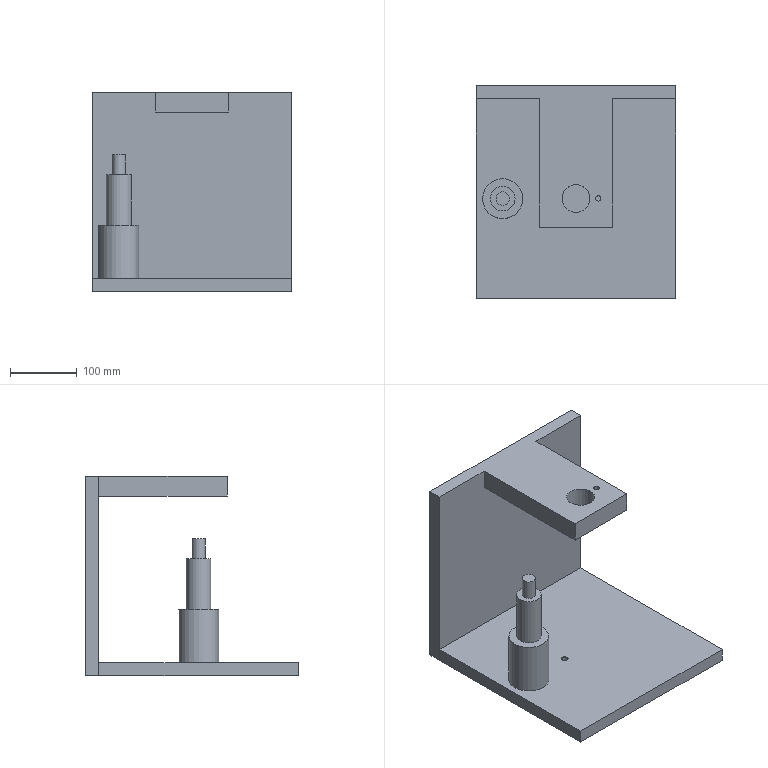Part | NX | features DATUM_CSYS 16, SKETCH 15, EXTRUDE 6, SYMBOLIC_THREAD 2, HOLE PACKAGE 1, SIMPLE HOLE 1 | 2 solids | 27 faces | box 300 x 320 x 300 mm | volume 4510024 mm3 | plane 19 | cylinder 6 | cone 2 | commonest cylinder face diameters 8 x1 8.5 x1 20 x1 37 x1 42 x1 60 x1
STEP:
#1=CARTESIAN_POINT('',(-150.,150.,0.));
#2=VERTEX_POINT('',#1);
#3=CARTESIAN_POINT('',(-150.,-150.,0.));
#4=VERTEX_POINT('',#3);
#5=CARTESIAN_POINT('',(-150.,150.,0.));
#6=DIRECTION('',(0.,-1.,0.));
#7=VECTOR('',#6,1000.);
#8=LINE('',#5,#7);
#9=EDGE_CURVE('',#2,#4,#8,.T.);
#10=ORIENTED_EDGE('',*,*,#9,.T.);
#11=CARTESIAN_POINT('',(-150.,-150.,20.));
#12=VERTEX_POINT('',#11);
#13=CARTESIAN_POINT('',(-150.,-150.,20.));
#14=DIRECTION('',(0.,0.,-1.));
#15=VECTOR('',#14,1000.);
#16=LINE('',#13,#15);
#17=EDGE_CURVE('',#12,#4,#16,.T.);
#18=ORIENTED_EDGE('',*,*,#17,.F.);
#19=CARTESIAN_POINT('',(-150.,150.,20.));
#20=VERTEX_POINT('',#19);
#21=CARTESIAN_POINT('',(-150.,150.,20.));
#22=DIRECTION('',(0.,-1.,0.));
#23=VECTOR('',#22,1000.);
#24=LINE('',#21,#23);
#25=EDGE_CURVE('',#20,#12,#24,.T.);
#26=ORIENTED_EDGE('',*,*,#25,.F.);
#27=CARTESIAN_POINT('',(-150.,150.,20.));
#28=DIRECTION('',(0.,0.,-1.));
#29=VECTOR('',#28,1000.);
#30=LINE('',#27,#29);
#31=EDGE_CURVE('',#20,#2,#30,.T.);
#32=ORIENTED_EDGE('',*,*,#31,.T.);
#33=EDGE_LOOP('',(#10,#18,#26,#32));
#34=FACE_BOUND('',#33,.T.);
#35=CARTESIAN_POINT('',(-150.,150.,20.));
#36=DIRECTION('',(1.,0.,0.));
#37=DIRECTION('',(0.,1.,0.));
#38=AXIS2_PLACEMENT_3D('',#35,#36,#37);
#39=PLANE('',#38);
#40=ADVANCED_FACE('',(#34),#39,.F.);
#41=CARTESIAN_POINT('',(150.,-150.,0.));
#42=VERTEX_POINT('',#41);
#43=CARTESIAN_POINT('',(-150.,-150.,0.));
#44=DIRECTION('',(1.,0.,0.));
#45=VECTOR('',#44,1000.);
#46=LINE('',#43,#45);
#47=EDGE_CURVE('',#4,#42,#46,.T.);
#48=ORIENTED_EDGE('',*,*,#47,.T.);
#49=CARTESIAN_POINT('',(150.,-150.,20.));
#50=VERTEX_POINT('',#49);
#51=CARTESIAN_POINT('',(150.,-150.,20.));
#52=DIRECTION('',(0.,0.,-1.));
#53=VECTOR('',#52,1000.);
#54=LINE('',#51,#53);
#55=EDGE_CURVE('',#50,#42,#54,.T.);
#56=ORIENTED_EDGE('',*,*,#55,.F.);
#57=CARTESIAN_POINT('',(-150.,-150.,20.));
#58=DIRECTION('',(1.,0.,0.));
#59=VECTOR('',#58,1000.);
#60=LINE('',#57,#59);
#61=EDGE_CURVE('',#12,#50,#60,.T.);
#62=ORIENTED_EDGE('',*,*,#61,.F.);
#63=ORIENTED_EDGE('',*,*,#17,.T.);
#64=EDGE_LOOP('',(#48,#56,#62,#63));
#65=FACE_BOUND('',#64,.T.);
#66=CARTESIAN_POINT('',(-150.,-150.,20.));
#67=DIRECTION('',(0.,1.,0.));
#68=DIRECTION('',(0.,0.,1.));
#69=AXIS2_PLACEMENT_3D('',#66,#67,#68);
#70=PLANE('',#69);
#71=ADVANCED_FACE('',(#65),#70,.F.);
#72=CARTESIAN_POINT('',(150.,150.,0.));
#73=VERTEX_POINT('',#72);
#74=CARTESIAN_POINT('',(150.,-150.,0.));
#75=DIRECTION('',(0.,1.,0.));
#76=VECTOR('',#75,1000.);
#77=LINE('',#74,#76);
#78=EDGE_CURVE('',#42,#73,#77,.T.);
#79=ORIENTED_EDGE('',*,*,#78,.T.);
#80=CARTESIAN_POINT('',(150.,150.,20.));
#81=VERTEX_POINT('',#80);
#82=CARTESIAN_POINT('',(150.,150.,20.));
#83=DIRECTION('',(0.,0.,-1.));
#84=VECTOR('',#83,1000.);
#85=LINE('',#82,#84);
#86=EDGE_CURVE('',#81,#73,#85,.T.);
#87=ORIENTED_EDGE('',*,*,#86,.F.);
#88=CARTESIAN_POINT('',(150.,-150.,20.));
#89=DIRECTION('',(0.,1.,0.));
#90=VECTOR('',#89,1000.);
#91=LINE('',#88,#90);
#92=EDGE_CURVE('',#50,#81,#91,.T.);
#93=ORIENTED_EDGE('',*,*,#92,.F.);
#94=ORIENTED_EDGE('',*,*,#55,.T.);
#95=EDGE_LOOP('',(#79,#87,#93,#94));
#96=FACE_BOUND('',#95,.T.);
#97=CARTESIAN_POINT('',(150.,-150.,20.));
#98=DIRECTION('',(-1.,0.,0.));
#99=DIRECTION('',(0.,-1.,0.));
#100=AXIS2_PLACEMENT_3D('',#97,#98,#99);
#101=PLANE('',#100);
#102=ADVANCED_FACE('',(#96),#101,.F.);
#103=CARTESIAN_POINT('',(150.,150.,0.));
#104=DIRECTION('',(-1.,0.,0.));
#105=VECTOR('',#104,1000.);
#106=LINE('',#103,#105);
#107=EDGE_CURVE('',#73,#2,#106,.T.);
#108=ORIENTED_EDGE('',*,*,#107,.T.);
#109=ORIENTED_EDGE('',*,*,#31,.F.);
#110=CARTESIAN_POINT('',(150.,150.,20.));
#111=DIRECTION('',(-1.,0.,0.));
#112=VECTOR('',#111,1000.);
#113=LINE('',#110,#112);
#114=EDGE_CURVE('',#81,#20,#113,.T.);
#115=ORIENTED_EDGE('',*,*,#114,.F.);
#116=ORIENTED_EDGE('',*,*,#86,.T.);
#117=EDGE_LOOP('',(#108,#109,#115,#116));
#118=FACE_BOUND('',#117,.T.);
#119=CARTESIAN_POINT('',(150.,150.,20.));
#120=DIRECTION('',(0.,-1.,0.));
#121=DIRECTION('',(0.,0.,-1.));
#122=AXIS2_PLACEMENT_3D('',#119,#120,#121);
#123=PLANE('',#122);
#124=ADVANCED_FACE('',(#118),#123,.F.);
#125=CARTESIAN_POINT('',(-29.,0.,20.));
#126=VERTEX_POINT('',#125);
#127=CARTESIAN_POINT('',(-34.,0.,20.));
#128=DIRECTION('',(0.,0.,1.));
#129=DIRECTION('',(1.,0.,0.));
#130=AXIS2_PLACEMENT_3D('',#127,#128,#129);
#131=CIRCLE('',#130,5.);
#132=EDGE_CURVE('',#126,#126,#131,.F.);
#133=ORIENTED_EDGE('',*,*,#132,.T.);
#134=EDGE_LOOP('',(#133));
#135=FACE_BOUND('',#134,.T.);
#136=CARTESIAN_POINT('',(-80.,0.,20.));
#137=VERTEX_POINT('',#136);
#138=CARTESIAN_POINT('',(-110.,0.,20.));
#139=DIRECTION('',(0.,0.,1.));
#140=DIRECTION('',(1.,0.,0.));
#141=AXIS2_PLACEMENT_3D('',#138,#139,#140);
#142=CIRCLE('',#141,30.);
#143=EDGE_CURVE('',#137,#137,#142,.F.);
#144=ORIENTED_EDGE('',*,*,#143,.T.);
#145=EDGE_LOOP('',(#144));
#146=FACE_BOUND('',#145,.T.);
#147=ORIENTED_EDGE('',*,*,#25,.T.);
#148=ORIENTED_EDGE('',*,*,#61,.T.);
#149=ORIENTED_EDGE('',*,*,#92,.T.);
#150=ORIENTED_EDGE('',*,*,#114,.T.);
#151=EDGE_LOOP('',(#147,#148,#149,#150));
#152=FACE_BOUND('',#151,.T.);
#153=CARTESIAN_POINT('',(0.,0.,20.));
#154=DIRECTION('',(0.,0.,1.));
#155=DIRECTION('',(1.,0.,0.));
#156=AXIS2_PLACEMENT_3D('',#153,#154,#155);
#157=PLANE('',#156);
#158=ADVANCED_FACE('',(#135,#146,#152),#157,.T.);
#159=ORIENTED_EDGE('',*,*,#9,.F.);
#160=ORIENTED_EDGE('',*,*,#107,.F.);
#161=ORIENTED_EDGE('',*,*,#78,.F.);
#162=ORIENTED_EDGE('',*,*,#47,.F.);
#163=EDGE_LOOP('',(#159,#160,#161,#162));
#164=FACE_BOUND('',#163,.T.);
#165=CARTESIAN_POINT('',(0.,0.,0.));
#166=DIRECTION('',(0.,0.,1.));
#167=DIRECTION('',(1.,0.,0.));
#168=AXIS2_PLACEMENT_3D('',#165,#166,#167);
#169=PLANE('',#168);
#170=ADVANCED_FACE('',(#164),#169,.F.);
#171=ORIENTED_EDGE('',*,*,#143,.F.);
#172=EDGE_LOOP('',(#171));
#173=FACE_BOUND('',#172,.T.);
#174=CARTESIAN_POINT('',(-80.,0.,100.));
#175=VERTEX_POINT('',#174);
#176=CARTESIAN_POINT('',(-110.,0.,100.));
#177=DIRECTION('',(0.,0.,1.));
#178=DIRECTION('',(1.,0.,0.));
#179=AXIS2_PLACEMENT_3D('',#176,#177,#178);
#180=CIRCLE('',#179,30.);
#181=EDGE_CURVE('',#175,#175,#180,.T.);
#182=ORIENTED_EDGE('',*,*,#181,.F.);
#183=EDGE_LOOP('',(#182));
#184=FACE_BOUND('',#183,.T.);
#185=CARTESIAN_POINT('',(-110.,0.,100.));
#186=DIRECTION('',(0.,0.,-1.));
#187=DIRECTION('',(-1.,0.,0.));
#188=AXIS2_PLACEMENT_3D('',#185,#186,#187);
#189=CYLINDRICAL_SURFACE('',#188,30.);
#190=ADVANCED_FACE('',(#173,#184),#189,.T.);
#191=CARTESIAN_POINT('',(-91.5,0.,100.));
#192=VERTEX_POINT('',#191);
#193=CARTESIAN_POINT('',(-110.,0.,100.));
#194=DIRECTION('',(0.,0.,1.));
#195=DIRECTION('',(1.,0.,0.));
#196=AXIS2_PLACEMENT_3D('',#193,#194,#195);
#197=CIRCLE('',#196,18.5);
#198=EDGE_CURVE('',#192,#192,#197,.T.);
#199=ORIENTED_EDGE('',*,*,#198,.F.);
#200=EDGE_LOOP('',(#199));
#201=FACE_BOUND('',#200,.T.);
#202=ORIENTED_EDGE('',*,*,#181,.T.);
#203=EDGE_LOOP('',(#202));
#204=FACE_BOUND('',#203,.T.);
#205=CARTESIAN_POINT('',(-110.,0.,100.));
#206=DIRECTION('',(0.,0.,1.));
#207=DIRECTION('',(1.,0.,0.));
#208=AXIS2_PLACEMENT_3D('',#205,#206,#207);
#209=PLANE('',#208);
#210=ADVANCED_FACE('',(#201,#204),#209,.T.);
#211=CARTESIAN_POINT('',(-91.5,0.,176.));
#212=VERTEX_POINT('',#211);
#213=CARTESIAN_POINT('',(-110.,0.,176.));
#214=DIRECTION('',(0.,0.,1.));
#215=DIRECTION('',(1.,0.,0.));
#216=AXIS2_PLACEMENT_3D('',#213,#214,#215);
#217=CIRCLE('',#216,18.5);
#218=EDGE_CURVE('',#212,#212,#217,.T.);
#219=ORIENTED_EDGE('',*,*,#218,.F.);
#220=EDGE_LOOP('',(#219));
#221=FACE_BOUND('',#220,.T.);
#222=ORIENTED_EDGE('',*,*,#198,.T.);
#223=EDGE_LOOP('',(#222));
#224=FACE_BOUND('',#223,.T.);
#225=CARTESIAN_POINT('',(-110.,0.,176.));
#226=DIRECTION('',(0.,0.,-1.));
#227=DIRECTION('',(-1.,0.,0.));
#228=AXIS2_PLACEMENT_3D('',#225,#226,#227);
#229=CYLINDRICAL_SURFACE('',#228,18.5);
#230=ADVANCED_FACE('',(#221,#224),#229,.T.);
#231=CARTESIAN_POINT('',(-100.,0.,176.));
#232=VERTEX_POINT('',#231);
#233=CARTESIAN_POINT('',(-110.,0.,176.));
#234=DIRECTION('',(0.,0.,1.));
#235=DIRECTION('',(1.,0.,0.));
#236=AXIS2_PLACEMENT_3D('',#233,#234,#235);
#237=CIRCLE('',#236,10.);
#238=EDGE_CURVE('',#232,#232,#237,.T.);
#239=ORIENTED_EDGE('',*,*,#238,.F.);
#240=EDGE_LOOP('',(#239));
#241=FACE_BOUND('',#240,.T.);
#242=ORIENTED_EDGE('',*,*,#218,.T.);
#243=EDGE_LOOP('',(#242));
#244=FACE_BOUND('',#243,.T.);
#245=CARTESIAN_POINT('',(-110.,0.,176.));
#246=DIRECTION('',(0.,0.,1.));
#247=DIRECTION('',(1.,0.,0.));
#248=AXIS2_PLACEMENT_3D('',#245,#246,#247);
#249=PLANE('',#248);
#250=ADVANCED_FACE('',(#241,#244),#249,.T.);
#251=CARTESIAN_POINT('',(-100.,0.,206.));
#252=VERTEX_POINT('',#251);
#253=CARTESIAN_POINT('',(-110.,0.,206.));
#254=DIRECTION('',(0.,0.,1.));
#255=DIRECTION('',(1.,0.,0.));
#256=AXIS2_PLACEMENT_3D('',#253,#254,#255);
#257=CIRCLE('',#256,10.);
#258=EDGE_CURVE('',#252,#252,#257,.T.);
#259=ORIENTED_EDGE('',*,*,#258,.F.);
#260=EDGE_LOOP('',(#259));
#261=FACE_BOUND('',#260,.T.);
#262=ORIENTED_EDGE('',*,*,#238,.T.);
#263=EDGE_LOOP('',(#262));
#264=FACE_BOUND('',#263,.T.);
#265=CARTESIAN_POINT('',(-110.,0.,206.));
#266=DIRECTION('',(0.,0.,-1.));
#267=DIRECTION('',(-1.,0.,0.));
#268=AXIS2_PLACEMENT_3D('',#265,#266,#267);
#269=CYLINDRICAL_SURFACE('',#268,10.);
#270=ADVANCED_FACE('',(#261,#264),#269,.T.);
#271=ORIENTED_EDGE('',*,*,#258,.T.);
#272=EDGE_LOOP('',(#271));
#273=FACE_BOUND('',#272,.T.);
#274=CARTESIAN_POINT('',(-110.,0.,206.));
#275=DIRECTION('',(0.,0.,1.));
#276=DIRECTION('',(1.,0.,0.));
#277=AXIS2_PLACEMENT_3D('',#274,#275,#276);
#278=PLANE('',#277);
#279=ADVANCED_FACE('',(#273),#278,.T.);
#280=CARTESIAN_POINT('',(-38.25,0.,5.));
#281=VERTEX_POINT('',#280);
#282=CARTESIAN_POINT('',(-34.,0.,5.));
#283=DIRECTION('',(0.,0.,-1.));
#284=DIRECTION('',(-1.,0.,0.));
#285=AXIS2_PLACEMENT_3D('',#282,#283,#284);
#286=CIRCLE('',#285,4.25);
#287=EDGE_CURVE('',#281,#281,#286,.F.);
#288=ORIENTED_EDGE('',*,*,#287,.T.);
#289=EDGE_LOOP('',(#288));
#290=FACE_BOUND('',#289,.T.);
#291=CARTESIAN_POINT('',(-34.,0.,2.446));
#292=VERTEX_POINT('',#291);
#293=VERTEX_LOOP('',#292);
#294=FACE_BOUND('',#293,.T.);
#295=CARTESIAN_POINT('',(-34.,0.,5.));
#296=DIRECTION('',(0.,0.,1.));
#297=DIRECTION('',(1.,0.,0.));
#298=AXIS2_PLACEMENT_3D('',#295,#296,#297);
#299=CONICAL_SURFACE('',#298,4.25,1.03);
#300=ADVANCED_FACE('',(#290,#294),#299,.F.);
#301=CARTESIAN_POINT('',(-29.75,0.,19.25));
#302=VERTEX_POINT('',#301);
#303=CARTESIAN_POINT('',(-34.,0.,19.25));
#304=DIRECTION('',(0.,0.,1.));
#305=DIRECTION('',(1.,0.,0.));
#306=AXIS2_PLACEMENT_3D('',#303,#304,#305);
#307=CIRCLE('',#306,4.25);
#308=EDGE_CURVE('',#302,#302,#307,.T.);
#309=ORIENTED_EDGE('',*,*,#308,.T.);
#310=EDGE_LOOP('',(#309));
#311=FACE_BOUND('',#310,.T.);
#312=ORIENTED_EDGE('',*,*,#287,.F.);
#313=EDGE_LOOP('',(#312));
#314=FACE_BOUND('',#313,.T.);
#315=CARTESIAN_POINT('',(-34.,0.,20.));
#316=DIRECTION('',(0.,0.,-1.));
#317=DIRECTION('',(-1.,0.,0.));
#318=AXIS2_PLACEMENT_3D('',#315,#316,#317);
#319=CYLINDRICAL_SURFACE('',#318,4.25);
#320=ADVANCED_FACE('',(#311,#314),#319,.F.);
#321=ORIENTED_EDGE('',*,*,#308,.F.);
#322=EDGE_LOOP('',(#321));
#323=FACE_BOUND('',#322,.T.);
#324=ORIENTED_EDGE('',*,*,#132,.F.);
#325=EDGE_LOOP('',(#324));
#326=FACE_BOUND('',#325,.T.);
#327=CARTESIAN_POINT('',(-34.,0.,20.));
#328=DIRECTION('',(0.,0.,1.));
#329=DIRECTION('',(1.,0.,0.));
#330=AXIS2_PLACEMENT_3D('',#327,#328,#329);
#331=CONICAL_SURFACE('',#330,5.,0.7854);
#332=ADVANCED_FACE('',(#323,#326),#331,.F.);
#333=CLOSED_SHELL('',(#40,#71,#102,#124,#158,#170,#190,#210,#230,#250,#270,#279,#300,#320,#332));
#334=MANIFOLD_SOLID_BREP('',#333);
#335=CARTESIAN_POINT('',(-55.,150.,300.));
#336=VERTEX_POINT('',#335);
#337=CARTESIAN_POINT('',(-55.,150.,270.));
#338=VERTEX_POINT('',#337);
#339=CARTESIAN_POINT('',(-55.,150.,300.));
#340=DIRECTION('',(0.,0.,-1.));
#341=VECTOR('',#340,1000.);
#342=LINE('',#339,#341);
#343=EDGE_CURVE('',#336,#338,#342,.T.);
#344=ORIENTED_EDGE('',*,*,#343,.F.);
#345=CARTESIAN_POINT('',(-150.,150.,300.));
#346=VERTEX_POINT('',#345);
#347=CARTESIAN_POINT('',(-150.,150.,300.));
#348=DIRECTION('',(1.,0.,0.));
#349=VECTOR('',#348,1000.);
#350=LINE('',#347,#349);
#351=EDGE_CURVE('',#346,#336,#350,.T.);
#352=ORIENTED_EDGE('',*,*,#351,.F.);
#353=CARTESIAN_POINT('',(-150.,150.,0.));
#354=VERTEX_POINT('',#353);
#355=CARTESIAN_POINT('',(-150.,150.,300.));
#356=DIRECTION('',(0.,0.,-1.));
#357=VECTOR('',#356,1000.);
#358=LINE('',#355,#357);
#359=EDGE_CURVE('',#346,#354,#358,.T.);
#360=ORIENTED_EDGE('',*,*,#359,.T.);
#361=CARTESIAN_POINT('',(150.,150.,0.));
#362=VERTEX_POINT('',#361);
#363=CARTESIAN_POINT('',(-150.,150.,0.));
#364=DIRECTION('',(1.,0.,0.));
#365=VECTOR('',#364,1000.);
#366=LINE('',#363,#365);
#367=EDGE_CURVE('',#354,#362,#366,.T.);
#368=ORIENTED_EDGE('',*,*,#367,.T.);
#369=CARTESIAN_POINT('',(150.,150.,300.));
#370=VERTEX_POINT('',#369);
#371=CARTESIAN_POINT('',(150.,150.,300.));
#372=DIRECTION('',(0.,0.,-1.));
#373=VECTOR('',#372,1000.);
#374=LINE('',#371,#373);
#375=EDGE_CURVE('',#370,#362,#374,.T.);
#376=ORIENTED_EDGE('',*,*,#375,.F.);
#377=CARTESIAN_POINT('',(55.,150.,300.));
#378=VERTEX_POINT('',#377);
#379=CARTESIAN_POINT('',(-150.,150.,300.));
#380=DIRECTION('',(1.,0.,0.));
#381=VECTOR('',#380,1000.);
#382=LINE('',#379,#381);
#383=EDGE_CURVE('',#378,#370,#382,.T.);
#384=ORIENTED_EDGE('',*,*,#383,.F.);
#385=CARTESIAN_POINT('',(55.,150.,270.));
#386=VERTEX_POINT('',#385);
#387=CARTESIAN_POINT('',(55.,150.,300.));
#388=DIRECTION('',(0.,0.,1.));
#389=VECTOR('',#388,1000.);
#390=LINE('',#387,#389);
#391=EDGE_CURVE('',#386,#378,#390,.T.);
#392=ORIENTED_EDGE('',*,*,#391,.F.);
#393=CARTESIAN_POINT('',(-150.,150.,270.));
#394=DIRECTION('',(1.,0.,0.));
#395=VECTOR('',#394,1000.);
#396=LINE('',#393,#395);
#397=EDGE_CURVE('',#338,#386,#396,.T.);
#398=ORIENTED_EDGE('',*,*,#397,.F.);
#399=EDGE_LOOP('',(#344,#352,#360,#368,#376,#384,#392,#398));
#400=FACE_BOUND('',#399,.T.);
#401=CARTESIAN_POINT('',(-150.,150.,300.));
#402=DIRECTION('',(0.,1.,0.));
#403=DIRECTION('',(0.,0.,1.));
#404=AXIS2_PLACEMENT_3D('',#401,#402,#403);
#405=PLANE('',#404);
#406=ADVANCED_FACE('',(#400),#405,.F.);
#407=CARTESIAN_POINT('',(-150.,170.,0.));
#408=VERTEX_POINT('',#407);
#409=CARTESIAN_POINT('',(-150.,170.,0.));
#410=DIRECTION('',(0.,-1.,0.));
#411=VECTOR('',#410,1000.);
#412=LINE('',#409,#411);
#413=EDGE_CURVE('',#408,#354,#412,.T.);
#414=ORIENTED_EDGE('',*,*,#413,.T.);
#415=ORIENTED_EDGE('',*,*,#359,.F.);
#416=CARTESIAN_POINT('',(-150.,170.,300.));
#417=VERTEX_POINT('',#416);
#418=CARTESIAN_POINT('',(-150.,170.,300.));
#419=DIRECTION('',(0.,-1.,0.));
#420=VECTOR('',#419,1000.);
#421=LINE('',#418,#420);
#422=EDGE_CURVE('',#417,#346,#421,.T.);
#423=ORIENTED_EDGE('',*,*,#422,.F.);
#424=CARTESIAN_POINT('',(-150.,170.,300.));
#425=DIRECTION('',(0.,0.,-1.));
#426=VECTOR('',#425,1000.);
#427=LINE('',#424,#426);
#428=EDGE_CURVE('',#417,#408,#427,.T.);
#429=ORIENTED_EDGE('',*,*,#428,.T.);
#430=EDGE_LOOP('',(#414,#415,#423,#429));
#431=FACE_BOUND('',#430,.T.);
#432=CARTESIAN_POINT('',(-150.,170.,300.));
#433=DIRECTION('',(1.,0.,0.));
#434=DIRECTION('',(0.,0.,-1.));
#435=AXIS2_PLACEMENT_3D('',#432,#433,#434);
#436=PLANE('',#435);
#437=ADVANCED_FACE('',(#431),#436,.F.);
#438=CARTESIAN_POINT('',(150.,170.,0.));
#439=VERTEX_POINT('',#438);
#440=CARTESIAN_POINT('',(150.,150.,0.));
#441=DIRECTION('',(0.,1.,0.));
#442=VECTOR('',#441,1000.);
#443=LINE('',#440,#442);
#444=EDGE_CURVE('',#362,#439,#443,.T.);
#445=ORIENTED_EDGE('',*,*,#444,.T.);
#446=CARTESIAN_POINT('',(150.,170.,300.));
#447=VERTEX_POINT('',#446);
#448=CARTESIAN_POINT('',(150.,170.,300.));
#449=DIRECTION('',(0.,0.,-1.));
#450=VECTOR('',#449,1000.);
#451=LINE('',#448,#450);
#452=EDGE_CURVE('',#447,#439,#451,.T.);
#453=ORIENTED_EDGE('',*,*,#452,.F.);
#454=CARTESIAN_POINT('',(150.,150.,300.));
#455=DIRECTION('',(0.,1.,0.));
#456=VECTOR('',#455,1000.);
#457=LINE('',#454,#456);
#458=EDGE_CURVE('',#370,#447,#457,.T.);
#459=ORIENTED_EDGE('',*,*,#458,.F.);
#460=ORIENTED_EDGE('',*,*,#375,.T.);
#461=EDGE_LOOP('',(#445,#453,#459,#460));
#462=FACE_BOUND('',#461,.T.);
#463=CARTESIAN_POINT('',(150.,150.,300.));
#464=DIRECTION('',(-1.,0.,0.));
#465=DIRECTION('',(0.,0.,1.));
#466=AXIS2_PLACEMENT_3D('',#463,#464,#465);
#467=PLANE('',#466);
#468=ADVANCED_FACE('',(#462),#467,.F.);
#469=ORIENTED_EDGE('',*,*,#428,.F.);
#470=CARTESIAN_POINT('',(150.,170.,300.));
#471=DIRECTION('',(-1.,0.,0.));
#472=VECTOR('',#471,1000.);
#473=LINE('',#470,#472);
#474=EDGE_CURVE('',#447,#417,#473,.T.);
#475=ORIENTED_EDGE('',*,*,#474,.F.);
#476=ORIENTED_EDGE('',*,*,#452,.T.);
#477=CARTESIAN_POINT('',(150.,170.,0.));
#478=DIRECTION('',(-1.,0.,0.));
#479=VECTOR('',#478,1000.);
#480=LINE('',#477,#479);
#481=EDGE_CURVE('',#439,#408,#480,.T.);
#482=ORIENTED_EDGE('',*,*,#481,.T.);
#483=EDGE_LOOP('',(#469,#475,#476,#482));
#484=FACE_BOUND('',#483,.T.);
#485=CARTESIAN_POINT('',(150.,170.,300.));
#486=DIRECTION('',(0.,-1.,0.));
#487=DIRECTION('',(0.,0.,-1.));
#488=AXIS2_PLACEMENT_3D('',#485,#486,#487);
#489=PLANE('',#488);
#490=ADVANCED_FACE('',(#484),#489,.F.);
#491=ORIENTED_EDGE('',*,*,#351,.T.);
#492=CARTESIAN_POINT('',(-55.,-42.929,300.));
#493=VERTEX_POINT('',#492);
#494=CARTESIAN_POINT('',(-55.,147.071,300.));
#495=DIRECTION('',(0.,1.,0.));
#496=VECTOR('',#495,1000.);
#497=LINE('',#494,#496);
#498=EDGE_CURVE('',#493,#336,#497,.T.);
#499=ORIENTED_EDGE('',*,*,#498,.F.);
#500=CARTESIAN_POINT('',(55.,-42.929,300.));
#501=VERTEX_POINT('',#500);
#502=CARTESIAN_POINT('',(55.,-42.929,300.));
#503=DIRECTION('',(-1.,0.,0.));
#504=VECTOR('',#503,1000.);
#505=LINE('',#502,#504);
#506=EDGE_CURVE('',#501,#493,#505,.T.);
#507=ORIENTED_EDGE('',*,*,#506,.F.);
#508=CARTESIAN_POINT('',(55.,170.,300.));
#509=DIRECTION('',(0.,-1.,0.));
#510=VECTOR('',#509,1000.);
#511=LINE('',#508,#510);
#512=EDGE_CURVE('',#378,#501,#511,.T.);
#513=ORIENTED_EDGE('',*,*,#512,.F.);
#514=ORIENTED_EDGE('',*,*,#383,.T.);
#515=ORIENTED_EDGE('',*,*,#458,.T.);
#516=ORIENTED_EDGE('',*,*,#474,.T.);
#517=ORIENTED_EDGE('',*,*,#422,.T.);
#518=EDGE_LOOP('',(#491,#499,#507,#513,#514,#515,#516,#517));
#519=FACE_BOUND('',#518,.T.);
#520=CARTESIAN_POINT('',(21.,0.,300.));
#521=VERTEX_POINT('',#520);
#522=CARTESIAN_POINT('',(0.,0.,300.));
#523=DIRECTION('',(0.,0.,1.));
#524=DIRECTION('',(1.,0.,0.));
#525=AXIS2_PLACEMENT_3D('',#522,#523,#524);
#526=CIRCLE('',#525,21.);
#527=EDGE_CURVE('',#521,#521,#526,.T.);
#528=ORIENTED_EDGE('',*,*,#527,.F.);
#529=EDGE_LOOP('',(#528));
#530=FACE_BOUND('',#529,.T.);
#531=CARTESIAN_POINT('',(37.5,0.,300.));
#532=VERTEX_POINT('',#531);
#533=CARTESIAN_POINT('',(33.5,0.,300.));
#534=DIRECTION('',(0.,0.,1.));
#535=DIRECTION('',(1.,0.,0.));
#536=AXIS2_PLACEMENT_3D('',#533,#534,#535);
#537=CIRCLE('',#536,4.);
#538=EDGE_CURVE('',#532,#532,#537,.T.);
#539=ORIENTED_EDGE('',*,*,#538,.F.);
#540=EDGE_LOOP('',(#539));
#541=FACE_BOUND('',#540,.T.);
#542=CARTESIAN_POINT('',(0.,0.,300.));
#543=DIRECTION('',(0.,0.,1.));
#544=DIRECTION('',(1.,0.,0.));
#545=AXIS2_PLACEMENT_3D('',#542,#543,#544);
#546=PLANE('',#545);
#547=ADVANCED_FACE('',(#519,#530,#541),#546,.T.);
#548=ORIENTED_EDGE('',*,*,#413,.F.);
#549=ORIENTED_EDGE('',*,*,#481,.F.);
#550=ORIENTED_EDGE('',*,*,#444,.F.);
#551=ORIENTED_EDGE('',*,*,#367,.F.);
#552=EDGE_LOOP('',(#548,#549,#550,#551));
#553=FACE_BOUND('',#552,.T.);
#554=CARTESIAN_POINT('',(0.,0.,0.));
#555=DIRECTION('',(0.,0.,1.));
#556=DIRECTION('',(1.,0.,0.));
#557=AXIS2_PLACEMENT_3D('',#554,#555,#556);
#558=PLANE('',#557);
#559=ADVANCED_FACE('',(#553),#558,.F.);
#560=ORIENTED_EDGE('',*,*,#498,.T.);
#561=ORIENTED_EDGE('',*,*,#343,.T.);
#562=CARTESIAN_POINT('',(-55.,-42.929,270.));
#563=VERTEX_POINT('',#562);
#564=CARTESIAN_POINT('',(-55.,-42.929,270.));
#565=DIRECTION('',(0.,1.,0.));
#566=VECTOR('',#565,1000.);
#567=LINE('',#564,#566);
#568=EDGE_CURVE('',#563,#338,#567,.T.);
#569=ORIENTED_EDGE('',*,*,#568,.F.);
#570=CARTESIAN_POINT('',(-55.,-42.929,270.));
#571=DIRECTION('',(0.,0.,1.));
#572=VECTOR('',#571,1000.);
#573=LINE('',#570,#572);
#574=EDGE_CURVE('',#563,#493,#573,.T.);
#575=ORIENTED_EDGE('',*,*,#574,.T.);
#576=EDGE_LOOP('',(#560,#561,#569,#575));
#577=FACE_BOUND('',#576,.T.);
#578=CARTESIAN_POINT('',(-55.,147.071,270.));
#579=DIRECTION('',(1.,0.,0.));
#580=DIRECTION('',(0.,0.,-1.));
#581=AXIS2_PLACEMENT_3D('',#578,#579,#580);
#582=PLANE('',#581);
#583=ADVANCED_FACE('',(#577),#582,.F.);
#584=CARTESIAN_POINT('',(55.,-42.929,270.));
#585=VERTEX_POINT('',#584);
#586=CARTESIAN_POINT('',(55.,147.071,270.));
#587=DIRECTION('',(0.,-1.,0.));
#588=VECTOR('',#587,1000.);
#589=LINE('',#586,#588);
#590=EDGE_CURVE('',#386,#585,#589,.T.);
#591=ORIENTED_EDGE('',*,*,#590,.F.);
#592=ORIENTED_EDGE('',*,*,#391,.T.);
#593=ORIENTED_EDGE('',*,*,#512,.T.);
#594=CARTESIAN_POINT('',(55.,-42.929,270.));
#595=DIRECTION('',(0.,0.,1.));
#596=VECTOR('',#595,1000.);
#597=LINE('',#594,#596);
#598=EDGE_CURVE('',#585,#501,#597,.T.);
#599=ORIENTED_EDGE('',*,*,#598,.F.);
#600=EDGE_LOOP('',(#591,#592,#593,#599));
#601=FACE_BOUND('',#600,.T.);
#602=CARTESIAN_POINT('',(55.,170.,270.));
#603=DIRECTION('',(-1.,0.,0.));
#604=DIRECTION('',(0.,-1.,0.));
#605=AXIS2_PLACEMENT_3D('',#602,#603,#604);
#606=PLANE('',#605);
#607=ADVANCED_FACE('',(#601),#606,.F.);
#608=CARTESIAN_POINT('',(37.5,0.,270.));
#609=VERTEX_POINT('',#608);
#610=CARTESIAN_POINT('',(33.5,0.,270.));
#611=DIRECTION('',(0.,0.,1.));
#612=DIRECTION('',(1.,0.,0.));
#613=AXIS2_PLACEMENT_3D('',#610,#611,#612);
#614=CIRCLE('',#613,4.);
#615=EDGE_CURVE('',#609,#609,#614,.T.);
#616=ORIENTED_EDGE('',*,*,#615,.T.);
#617=EDGE_LOOP('',(#616));
#618=FACE_BOUND('',#617,.T.);
#619=CARTESIAN_POINT('',(21.,0.,270.));
#620=VERTEX_POINT('',#619);
#621=CARTESIAN_POINT('',(0.,0.,270.));
#622=DIRECTION('',(0.,0.,1.));
#623=DIRECTION('',(1.,0.,0.));
#624=AXIS2_PLACEMENT_3D('',#621,#622,#623);
#625=CIRCLE('',#624,21.);
#626=EDGE_CURVE('',#620,#620,#625,.T.);
#627=ORIENTED_EDGE('',*,*,#626,.T.);
#628=EDGE_LOOP('',(#627));
#629=FACE_BOUND('',#628,.T.);
#630=ORIENTED_EDGE('',*,*,#568,.T.);
#631=ORIENTED_EDGE('',*,*,#397,.T.);
#632=ORIENTED_EDGE('',*,*,#590,.T.);
#633=CARTESIAN_POINT('',(55.,-42.929,270.));
#634=DIRECTION('',(-1.,0.,0.));
#635=VECTOR('',#634,1000.);
#636=LINE('',#633,#635);
#637=EDGE_CURVE('',#585,#563,#636,.T.);
#638=ORIENTED_EDGE('',*,*,#637,.T.);
#639=EDGE_LOOP('',(#630,#631,#632,#638));
#640=FACE_BOUND('',#639,.T.);
#641=CARTESIAN_POINT('',(33.5,0.,270.));
#642=DIRECTION('',(0.,0.,1.));
#643=DIRECTION('',(1.,0.,0.));
#644=AXIS2_PLACEMENT_3D('',#641,#642,#643);
#645=PLANE('',#644);
#646=ADVANCED_FACE('',(#618,#629,#640),#645,.F.);
#647=ORIENTED_EDGE('',*,*,#506,.T.);
#648=ORIENTED_EDGE('',*,*,#574,.F.);
#649=ORIENTED_EDGE('',*,*,#637,.F.);
#650=ORIENTED_EDGE('',*,*,#598,.T.);
#651=EDGE_LOOP('',(#647,#648,#649,#650));
#652=FACE_BOUND('',#651,.T.);
#653=CARTESIAN_POINT('',(55.,-42.929,270.));
#654=DIRECTION('',(0.,1.,0.));
#655=DIRECTION('',(-1.,0.,0.));
#656=AXIS2_PLACEMENT_3D('',#653,#654,#655);
#657=PLANE('',#656);
#658=ADVANCED_FACE('',(#652),#657,.F.);
#659=ORIENTED_EDGE('',*,*,#615,.F.);
#660=EDGE_LOOP('',(#659));
#661=FACE_BOUND('',#660,.T.);
#662=ORIENTED_EDGE('',*,*,#538,.T.);
#663=EDGE_LOOP('',(#662));
#664=FACE_BOUND('',#663,.T.);
#665=CARTESIAN_POINT('',(33.5,0.,270.));
#666=DIRECTION('',(0.,0.,1.));
#667=DIRECTION('',(1.,0.,0.));
#668=AXIS2_PLACEMENT_3D('',#665,#666,#667);
#669=CYLINDRICAL_SURFACE('',#668,4.);
#670=ADVANCED_FACE('',(#661,#664),#669,.F.);
#671=ORIENTED_EDGE('',*,*,#626,.F.);
#672=EDGE_LOOP('',(#671));
#673=FACE_BOUND('',#672,.T.);
#674=ORIENTED_EDGE('',*,*,#527,.T.);
#675=EDGE_LOOP('',(#674));
#676=FACE_BOUND('',#675,.T.);
#677=CARTESIAN_POINT('',(0.,0.,270.));
#678=DIRECTION('',(0.,0.,1.));
#679=DIRECTION('',(1.,0.,0.));
#680=AXIS2_PLACEMENT_3D('',#677,#678,#679);
#681=CYLINDRICAL_SURFACE('',#680,21.);
#682=ADVANCED_FACE('',(#673,#676),#681,.F.);
#683=CLOSED_SHELL('',(#406,#437,#468,#490,#547,#559,#583,#607,#646,#658,#670,#682));
#684=MANIFOLD_SOLID_BREP('',#683);
#685=(LENGTH_UNIT()NAMED_UNIT(*)SI_UNIT(.MILLI.,.METRE.));
#686=UNCERTAINTY_MEASURE_WITH_UNIT(LENGTH_MEASURE(0.00001),#685,'','');
#687=(NAMED_UNIT(*)PLANE_ANGLE_UNIT()SI_UNIT($,.RADIAN.));
#688=(NAMED_UNIT(*)SI_UNIT($,.STERADIAN.)SOLID_ANGLE_UNIT());
#689=(GEOMETRIC_REPRESENTATION_CONTEXT(3)GLOBAL_UNCERTAINTY_ASSIGNED_CONTEXT((#686))GLOBAL_UNIT_ASSIGNED_CONTEXT((#685,#687,#688))REPRESENTATION_CONTEXT('',''));
#690=ADVANCED_BREP_SHAPE_REPRESENTATION('',(#334,#684),#689);